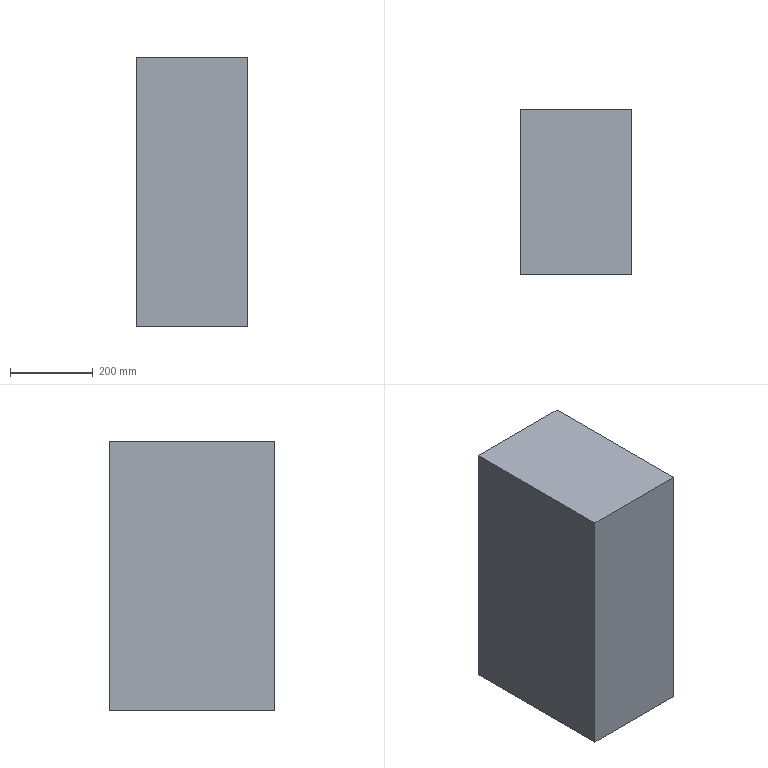Part | STEP file | kunzaxiang2 | 1 solid | 11 faces | box 270 x 400 x 650 mm | volume 28248000 mm3 | plane 11
STEP:
#1=CARTESIAN_POINT('',(0.,0.,0.));
#2=DIRECTION('',(0.,0.,1.));
#3=DIRECTION('',(1.,0.,0.));
#4=AXIS2_PLACEMENT_3D('',#1,#2,#3);
#5=CARTESIAN_POINT('',(135.,200.,325.));
#6=VERTEX_POINT('',#5);
#7=CARTESIAN_POINT('',(135.,200.,-325.));
#8=VERTEX_POINT('',#7);
#9=CARTESIAN_POINT('',(135.,200.,-325.));
#10=DIRECTION('',(0.,0.,-1.));
#11=VECTOR('',#10,1.);
#12=LINE('',#9,#11);
#13=CARTESIAN_POINT('',(0.,200.,0.));
#14=DIRECTION('',(0.,1.,0.));
#15=DIRECTION('',(0.,0.,1.));
#16=AXIS2_PLACEMENT_3D('',#13,#14,#15);
#17=PLANE('',#16);
#18=CARTESIAN_POINT('',(-325.,135.));
#19=DIRECTION('',(-1.,0.));
#20=VECTOR('',#19,1.);
#21=LINE('',#18,#20);
#22=(GEOMETRIC_REPRESENTATION_CONTEXT(2)PARAMETRIC_REPRESENTATION_CONTEXT()REPRESENTATION_CONTEXT('',''));
#23=DEFINITIONAL_REPRESENTATION('',(#21),#22);
#24=PCURVE('',#17,#23);
#25=CARTESIAN_POINT('',(135.,-200.,-325.));
#26=DIRECTION('',(1.,0.,0.));
#27=DIRECTION('',(0.,0.,-1.));
#28=AXIS2_PLACEMENT_3D('',#25,#26,#27);
#29=PLANE('',#28);
#30=CARTESIAN_POINT('',(0.,400.));
#31=DIRECTION('',(1.,0.));
#32=VECTOR('',#31,1.);
#33=LINE('',#30,#32);
#34=(GEOMETRIC_REPRESENTATION_CONTEXT(2)PARAMETRIC_REPRESENTATION_CONTEXT()REPRESENTATION_CONTEXT('',''));
#35=DEFINITIONAL_REPRESENTATION('',(#33),#34);
#36=PCURVE('',#29,#35);
#37=SURFACE_CURVE('',#12,(#24,#36),.PCURVE_S1.);
#38=EDGE_CURVE('',#6,#8,#37,.T.);
#39=ORIENTED_EDGE('',*,*,#38,.T.);
#40=CARTESIAN_POINT('',(-135.,200.,-325.));
#41=VERTEX_POINT('',#40);
#42=CARTESIAN_POINT('',(-135.,200.,-325.));
#43=DIRECTION('',(-1.,0.,0.));
#44=VECTOR('',#43,1.);
#45=LINE('',#42,#44);
#46=CARTESIAN_POINT('',(-325.,-135.));
#47=DIRECTION('',(0.,-1.));
#48=VECTOR('',#47,1.);
#49=LINE('',#46,#48);
#50=(GEOMETRIC_REPRESENTATION_CONTEXT(2)PARAMETRIC_REPRESENTATION_CONTEXT()REPRESENTATION_CONTEXT('',''));
#51=DEFINITIONAL_REPRESENTATION('',(#49),#50);
#52=PCURVE('',#17,#51);
#53=CARTESIAN_POINT('',(-135.,-200.,-325.));
#54=DIRECTION('',(0.,0.,-1.));
#55=DIRECTION('',(-1.,0.,0.));
#56=AXIS2_PLACEMENT_3D('',#53,#54,#55);
#57=PLANE('',#56);
#58=CARTESIAN_POINT('',(0.,400.));
#59=DIRECTION('',(1.,0.));
#60=VECTOR('',#59,1.);
#61=LINE('',#58,#60);
#62=(GEOMETRIC_REPRESENTATION_CONTEXT(2)PARAMETRIC_REPRESENTATION_CONTEXT()REPRESENTATION_CONTEXT('',''));
#63=DEFINITIONAL_REPRESENTATION('',(#61),#62);
#64=PCURVE('',#57,#63);
#65=SURFACE_CURVE('',#45,(#52,#64),.PCURVE_S1.);
#66=EDGE_CURVE('',#8,#41,#65,.T.);
#67=ORIENTED_EDGE('',*,*,#66,.T.);
#68=CARTESIAN_POINT('',(-135.,200.,325.));
#69=VERTEX_POINT('',#68);
#70=CARTESIAN_POINT('',(-135.,200.,-325.));
#71=DIRECTION('',(0.,0.,1.));
#72=VECTOR('',#71,1.);
#73=LINE('',#70,#72);
#74=CARTESIAN_POINT('',(-325.,-135.));
#75=DIRECTION('',(1.,0.));
#76=VECTOR('',#75,1.);
#77=LINE('',#74,#76);
#78=(GEOMETRIC_REPRESENTATION_CONTEXT(2)PARAMETRIC_REPRESENTATION_CONTEXT()REPRESENTATION_CONTEXT('',''));
#79=DEFINITIONAL_REPRESENTATION('',(#77),#78);
#80=PCURVE('',#17,#79);
#81=CARTESIAN_POINT('',(-135.,-200.,-325.));
#82=DIRECTION('',(-1.,0.,0.));
#83=DIRECTION('',(0.,0.,1.));
#84=AXIS2_PLACEMENT_3D('',#81,#82,#83);
#85=PLANE('',#84);
#86=CARTESIAN_POINT('',(0.,400.));
#87=DIRECTION('',(1.,0.));
#88=VECTOR('',#87,1.);
#89=LINE('',#86,#88);
#90=(GEOMETRIC_REPRESENTATION_CONTEXT(2)PARAMETRIC_REPRESENTATION_CONTEXT()REPRESENTATION_CONTEXT('',''));
#91=DEFINITIONAL_REPRESENTATION('',(#89),#90);
#92=PCURVE('',#85,#91);
#93=SURFACE_CURVE('',#73,(#80,#92),.PCURVE_S1.);
#94=EDGE_CURVE('',#41,#69,#93,.T.);
#95=ORIENTED_EDGE('',*,*,#94,.T.);
#96=CARTESIAN_POINT('',(-135.,200.,325.));
#97=DIRECTION('',(1.,0.,0.));
#98=VECTOR('',#97,1.);
#99=LINE('',#96,#98);
#100=CARTESIAN_POINT('',(325.,-135.));
#101=DIRECTION('',(0.,1.));
#102=VECTOR('',#101,1.);
#103=LINE('',#100,#102);
#104=(GEOMETRIC_REPRESENTATION_CONTEXT(2)PARAMETRIC_REPRESENTATION_CONTEXT()REPRESENTATION_CONTEXT('',''));
#105=DEFINITIONAL_REPRESENTATION('',(#103),#104);
#106=PCURVE('',#17,#105);
#107=CARTESIAN_POINT('',(-135.,-200.,325.));
#108=DIRECTION('',(0.,0.,1.));
#109=DIRECTION('',(1.,0.,0.));
#110=AXIS2_PLACEMENT_3D('',#107,#108,#109);
#111=PLANE('',#110);
#112=CARTESIAN_POINT('',(0.,400.));
#113=DIRECTION('',(1.,0.));
#114=VECTOR('',#113,1.);
#115=LINE('',#112,#114);
#116=(GEOMETRIC_REPRESENTATION_CONTEXT(2)PARAMETRIC_REPRESENTATION_CONTEXT()REPRESENTATION_CONTEXT('',''));
#117=DEFINITIONAL_REPRESENTATION('',(#115),#116);
#118=PCURVE('',#111,#117);
#119=SURFACE_CURVE('',#99,(#106,#118),.PCURVE_S1.);
#120=EDGE_CURVE('',#69,#6,#119,.T.);
#121=ORIENTED_EDGE('',*,*,#120,.T.);
#122=EDGE_LOOP('',(#39,#67,#95,#121));
#123=FACE_BOUND('',#122,.T.);
#124=CARTESIAN_POINT('',(120.,200.,-230.));
#125=VERTEX_POINT('',#124);
#126=CARTESIAN_POINT('',(-120.,200.,-230.));
#127=VERTEX_POINT('',#126);
#128=CARTESIAN_POINT('',(-120.,200.,-230.));
#129=DIRECTION('',(-1.,0.,0.));
#130=VECTOR('',#129,1.);
#131=LINE('',#128,#130);
#132=CARTESIAN_POINT('',(-230.,-120.));
#133=DIRECTION('',(0.,-1.));
#134=VECTOR('',#133,1.);
#135=LINE('',#132,#134);
#136=(GEOMETRIC_REPRESENTATION_CONTEXT(2)PARAMETRIC_REPRESENTATION_CONTEXT()REPRESENTATION_CONTEXT('',''));
#137=DEFINITIONAL_REPRESENTATION('',(#135),#136);
#138=PCURVE('',#17,#137);
#139=CARTESIAN_POINT('',(-120.,200.,-230.));
#140=DIRECTION('',(0.,0.,1.));
#141=DIRECTION('',(1.,0.,0.));
#142=AXIS2_PLACEMENT_3D('',#139,#140,#141);
#143=PLANE('',#142);
#144=CARTESIAN_POINT('',(0.,0.));
#145=DIRECTION('',(-1.,0.));
#146=VECTOR('',#145,1.);
#147=LINE('',#144,#146);
#148=(GEOMETRIC_REPRESENTATION_CONTEXT(2)PARAMETRIC_REPRESENTATION_CONTEXT()REPRESENTATION_CONTEXT('',''));
#149=DEFINITIONAL_REPRESENTATION('',(#147),#148);
#150=PCURVE('',#143,#149);
#151=SURFACE_CURVE('',#131,(#138,#150),.PCURVE_S1.);
#152=EDGE_CURVE('',#125,#127,#151,.T.);
#153=ORIENTED_EDGE('',*,*,#152,.F.);
#154=CARTESIAN_POINT('',(120.,200.,230.));
#155=VERTEX_POINT('',#154);
#156=CARTESIAN_POINT('',(120.,200.,-230.));
#157=DIRECTION('',(0.,0.,-1.));
#158=VECTOR('',#157,1.);
#159=LINE('',#156,#158);
#160=CARTESIAN_POINT('',(-230.,120.));
#161=DIRECTION('',(-1.,0.));
#162=VECTOR('',#161,1.);
#163=LINE('',#160,#162);
#164=(GEOMETRIC_REPRESENTATION_CONTEXT(2)PARAMETRIC_REPRESENTATION_CONTEXT()REPRESENTATION_CONTEXT('',''));
#165=DEFINITIONAL_REPRESENTATION('',(#163),#164);
#166=PCURVE('',#17,#165);
#167=CARTESIAN_POINT('',(120.,200.,-230.));
#168=DIRECTION('',(-1.,0.,0.));
#169=DIRECTION('',(0.,0.,1.));
#170=AXIS2_PLACEMENT_3D('',#167,#168,#169);
#171=PLANE('',#170);
#172=CARTESIAN_POINT('',(0.,0.));
#173=DIRECTION('',(-1.,0.));
#174=VECTOR('',#173,1.);
#175=LINE('',#172,#174);
#176=(GEOMETRIC_REPRESENTATION_CONTEXT(2)PARAMETRIC_REPRESENTATION_CONTEXT()REPRESENTATION_CONTEXT('',''));
#177=DEFINITIONAL_REPRESENTATION('',(#175),#176);
#178=PCURVE('',#171,#177);
#179=SURFACE_CURVE('',#159,(#166,#178),.PCURVE_S1.);
#180=EDGE_CURVE('',#155,#125,#179,.T.);
#181=ORIENTED_EDGE('',*,*,#180,.F.);
#182=CARTESIAN_POINT('',(-120.,200.,230.));
#183=VERTEX_POINT('',#182);
#184=CARTESIAN_POINT('',(-120.,200.,230.));
#185=DIRECTION('',(1.,0.,0.));
#186=VECTOR('',#185,1.);
#187=LINE('',#184,#186);
#188=CARTESIAN_POINT('',(230.,-120.));
#189=DIRECTION('',(0.,1.));
#190=VECTOR('',#189,1.);
#191=LINE('',#188,#190);
#192=(GEOMETRIC_REPRESENTATION_CONTEXT(2)PARAMETRIC_REPRESENTATION_CONTEXT()REPRESENTATION_CONTEXT('',''));
#193=DEFINITIONAL_REPRESENTATION('',(#191),#192);
#194=PCURVE('',#17,#193);
#195=CARTESIAN_POINT('',(-120.,200.,230.));
#196=DIRECTION('',(0.,0.,-1.));
#197=DIRECTION('',(-1.,0.,0.));
#198=AXIS2_PLACEMENT_3D('',#195,#196,#197);
#199=PLANE('',#198);
#200=CARTESIAN_POINT('',(0.,0.));
#201=DIRECTION('',(-1.,0.));
#202=VECTOR('',#201,1.);
#203=LINE('',#200,#202);
#204=(GEOMETRIC_REPRESENTATION_CONTEXT(2)PARAMETRIC_REPRESENTATION_CONTEXT()REPRESENTATION_CONTEXT('',''));
#205=DEFINITIONAL_REPRESENTATION('',(#203),#204);
#206=PCURVE('',#199,#205);
#207=SURFACE_CURVE('',#187,(#194,#206),.PCURVE_S1.);
#208=EDGE_CURVE('',#183,#155,#207,.T.);
#209=ORIENTED_EDGE('',*,*,#208,.F.);
#210=CARTESIAN_POINT('',(-120.,200.,-230.));
#211=DIRECTION('',(0.,0.,1.));
#212=VECTOR('',#211,1.);
#213=LINE('',#210,#212);
#214=CARTESIAN_POINT('',(-230.,-120.));
#215=DIRECTION('',(1.,0.));
#216=VECTOR('',#215,1.);
#217=LINE('',#214,#216);
#218=(GEOMETRIC_REPRESENTATION_CONTEXT(2)PARAMETRIC_REPRESENTATION_CONTEXT()REPRESENTATION_CONTEXT('',''));
#219=DEFINITIONAL_REPRESENTATION('',(#217),#218);
#220=PCURVE('',#17,#219);
#221=CARTESIAN_POINT('',(-120.,200.,-230.));
#222=DIRECTION('',(1.,0.,0.));
#223=DIRECTION('',(0.,0.,-1.));
#224=AXIS2_PLACEMENT_3D('',#221,#222,#223);
#225=PLANE('',#224);
#226=CARTESIAN_POINT('',(0.,0.));
#227=DIRECTION('',(-1.,0.));
#228=VECTOR('',#227,1.);
#229=LINE('',#226,#228);
#230=(GEOMETRIC_REPRESENTATION_CONTEXT(2)PARAMETRIC_REPRESENTATION_CONTEXT()REPRESENTATION_CONTEXT('',''));
#231=DEFINITIONAL_REPRESENTATION('',(#229),#230);
#232=PCURVE('',#225,#231);
#233=SURFACE_CURVE('',#213,(#220,#232),.PCURVE_S1.);
#234=EDGE_CURVE('',#127,#183,#233,.T.);
#235=ORIENTED_EDGE('',*,*,#234,.F.);
#236=EDGE_LOOP('',(#153,#181,#209,#235));
#237=FACE_BOUND('',#236,.T.);
#238=ADVANCED_FACE('',(#123,#237),#17,.T.);
#239=ORIENTED_EDGE('',*,*,#38,.F.);
#240=CARTESIAN_POINT('',(135.,-200.,325.));
#241=VERTEX_POINT('',#240);
#242=CARTESIAN_POINT('',(135.,-200.,325.));
#243=DIRECTION('',(0.,1.,0.));
#244=VECTOR('',#243,1.);
#245=LINE('',#242,#244);
#246=CARTESIAN_POINT('',(-650.,0.));
#247=DIRECTION('',(0.,1.));
#248=VECTOR('',#247,1.);
#249=LINE('',#246,#248);
#250=(GEOMETRIC_REPRESENTATION_CONTEXT(2)PARAMETRIC_REPRESENTATION_CONTEXT()REPRESENTATION_CONTEXT('',''));
#251=DEFINITIONAL_REPRESENTATION('',(#249),#250);
#252=PCURVE('',#29,#251);
#253=CARTESIAN_POINT('',(270.,0.));
#254=DIRECTION('',(0.,1.));
#255=VECTOR('',#254,1.);
#256=LINE('',#253,#255);
#257=(GEOMETRIC_REPRESENTATION_CONTEXT(2)PARAMETRIC_REPRESENTATION_CONTEXT()REPRESENTATION_CONTEXT('',''));
#258=DEFINITIONAL_REPRESENTATION('',(#256),#257);
#259=PCURVE('',#111,#258);
#260=SURFACE_CURVE('',#245,(#252,#259),.PCURVE_S1.);
#261=EDGE_CURVE('',#241,#6,#260,.T.);
#262=ORIENTED_EDGE('',*,*,#261,.F.);
#263=CARTESIAN_POINT('',(135.,-200.,-325.));
#264=VERTEX_POINT('',#263);
#265=CARTESIAN_POINT('',(135.,-200.,-325.));
#266=DIRECTION('',(0.,0.,-1.));
#267=VECTOR('',#266,1.);
#268=LINE('',#265,#267);
#269=CARTESIAN_POINT('',(0.,0.));
#270=DIRECTION('',(1.,0.));
#271=VECTOR('',#270,1.);
#272=LINE('',#269,#271);
#273=(GEOMETRIC_REPRESENTATION_CONTEXT(2)PARAMETRIC_REPRESENTATION_CONTEXT()REPRESENTATION_CONTEXT('',''));
#274=DEFINITIONAL_REPRESENTATION('',(#272),#273);
#275=PCURVE('',#29,#274);
#276=CARTESIAN_POINT('',(0.,-200.,0.));
#277=DIRECTION('',(0.,1.,0.));
#278=DIRECTION('',(0.,0.,1.));
#279=AXIS2_PLACEMENT_3D('',#276,#277,#278);
#280=PLANE('',#279);
#281=CARTESIAN_POINT('',(-325.,135.));
#282=DIRECTION('',(-1.,0.));
#283=VECTOR('',#282,1.);
#284=LINE('',#281,#283);
#285=(GEOMETRIC_REPRESENTATION_CONTEXT(2)PARAMETRIC_REPRESENTATION_CONTEXT()REPRESENTATION_CONTEXT('',''));
#286=DEFINITIONAL_REPRESENTATION('',(#284),#285);
#287=PCURVE('',#280,#286);
#288=SURFACE_CURVE('',#268,(#275,#287),.PCURVE_S1.);
#289=EDGE_CURVE('',#241,#264,#288,.T.);
#290=ORIENTED_EDGE('',*,*,#289,.T.);
#291=CARTESIAN_POINT('',(135.,-200.,-325.));
#292=DIRECTION('',(0.,1.,0.));
#293=VECTOR('',#292,1.);
#294=LINE('',#291,#293);
#295=CARTESIAN_POINT('',(0.,0.));
#296=DIRECTION('',(0.,1.));
#297=VECTOR('',#296,1.);
#298=LINE('',#295,#297);
#299=(GEOMETRIC_REPRESENTATION_CONTEXT(2)PARAMETRIC_REPRESENTATION_CONTEXT()REPRESENTATION_CONTEXT('',''));
#300=DEFINITIONAL_REPRESENTATION('',(#298),#299);
#301=PCURVE('',#29,#300);
#302=CARTESIAN_POINT('',(-270.,0.));
#303=DIRECTION('',(0.,1.));
#304=VECTOR('',#303,1.);
#305=LINE('',#302,#304);
#306=(GEOMETRIC_REPRESENTATION_CONTEXT(2)PARAMETRIC_REPRESENTATION_CONTEXT()REPRESENTATION_CONTEXT('',''));
#307=DEFINITIONAL_REPRESENTATION('',(#305),#306);
#308=PCURVE('',#57,#307);
#309=SURFACE_CURVE('',#294,(#301,#308),.PCURVE_S1.);
#310=EDGE_CURVE('',#264,#8,#309,.T.);
#311=ORIENTED_EDGE('',*,*,#310,.T.);
#312=EDGE_LOOP('',(#239,#262,#290,#311));
#313=FACE_BOUND('',#312,.T.);
#314=ADVANCED_FACE('',(#313),#29,.T.);
#315=ORIENTED_EDGE('',*,*,#120,.F.);
#316=CARTESIAN_POINT('',(-135.,-200.,325.));
#317=VERTEX_POINT('',#316);
#318=CARTESIAN_POINT('',(-135.,-200.,325.));
#319=DIRECTION('',(0.,1.,0.));
#320=VECTOR('',#319,1.);
#321=LINE('',#318,#320);
#322=CARTESIAN_POINT('',(0.,0.));
#323=DIRECTION('',(0.,1.));
#324=VECTOR('',#323,1.);
#325=LINE('',#322,#324);
#326=(GEOMETRIC_REPRESENTATION_CONTEXT(2)PARAMETRIC_REPRESENTATION_CONTEXT()REPRESENTATION_CONTEXT('',''));
#327=DEFINITIONAL_REPRESENTATION('',(#325),#326);
#328=PCURVE('',#111,#327);
#329=CARTESIAN_POINT('',(650.,0.));
#330=DIRECTION('',(0.,1.));
#331=VECTOR('',#330,1.);
#332=LINE('',#329,#331);
#333=(GEOMETRIC_REPRESENTATION_CONTEXT(2)PARAMETRIC_REPRESENTATION_CONTEXT()REPRESENTATION_CONTEXT('',''));
#334=DEFINITIONAL_REPRESENTATION('',(#332),#333);
#335=PCURVE('',#85,#334);
#336=SURFACE_CURVE('',#321,(#328,#335),.PCURVE_S1.);
#337=EDGE_CURVE('',#317,#69,#336,.T.);
#338=ORIENTED_EDGE('',*,*,#337,.F.);
#339=CARTESIAN_POINT('',(-135.,-200.,325.));
#340=DIRECTION('',(1.,0.,0.));
#341=VECTOR('',#340,1.);
#342=LINE('',#339,#341);
#343=CARTESIAN_POINT('',(0.,0.));
#344=DIRECTION('',(1.,0.));
#345=VECTOR('',#344,1.);
#346=LINE('',#343,#345);
#347=(GEOMETRIC_REPRESENTATION_CONTEXT(2)PARAMETRIC_REPRESENTATION_CONTEXT()REPRESENTATION_CONTEXT('',''));
#348=DEFINITIONAL_REPRESENTATION('',(#346),#347);
#349=PCURVE('',#111,#348);
#350=CARTESIAN_POINT('',(325.,-135.));
#351=DIRECTION('',(0.,1.));
#352=VECTOR('',#351,1.);
#353=LINE('',#350,#352);
#354=(GEOMETRIC_REPRESENTATION_CONTEXT(2)PARAMETRIC_REPRESENTATION_CONTEXT()REPRESENTATION_CONTEXT('',''));
#355=DEFINITIONAL_REPRESENTATION('',(#353),#354);
#356=PCURVE('',#280,#355);
#357=SURFACE_CURVE('',#342,(#349,#356),.PCURVE_S1.);
#358=EDGE_CURVE('',#317,#241,#357,.T.);
#359=ORIENTED_EDGE('',*,*,#358,.T.);
#360=ORIENTED_EDGE('',*,*,#261,.T.);
#361=EDGE_LOOP('',(#315,#338,#359,#360));
#362=FACE_BOUND('',#361,.T.);
#363=ADVANCED_FACE('',(#362),#111,.T.);
#364=ORIENTED_EDGE('',*,*,#94,.F.);
#365=CARTESIAN_POINT('',(-135.,-200.,-325.));
#366=VERTEX_POINT('',#365);
#367=CARTESIAN_POINT('',(-135.,-200.,-325.));
#368=DIRECTION('',(0.,1.,0.));
#369=VECTOR('',#368,1.);
#370=LINE('',#367,#369);
#371=CARTESIAN_POINT('',(0.,0.));
#372=DIRECTION('',(0.,1.));
#373=VECTOR('',#372,1.);
#374=LINE('',#371,#373);
#375=(GEOMETRIC_REPRESENTATION_CONTEXT(2)PARAMETRIC_REPRESENTATION_CONTEXT()REPRESENTATION_CONTEXT('',''));
#376=DEFINITIONAL_REPRESENTATION('',(#374),#375);
#377=PCURVE('',#85,#376);
#378=CARTESIAN_POINT('',(0.,0.));
#379=DIRECTION('',(0.,1.));
#380=VECTOR('',#379,1.);
#381=LINE('',#378,#380);
#382=(GEOMETRIC_REPRESENTATION_CONTEXT(2)PARAMETRIC_REPRESENTATION_CONTEXT()REPRESENTATION_CONTEXT('',''));
#383=DEFINITIONAL_REPRESENTATION('',(#381),#382);
#384=PCURVE('',#57,#383);
#385=SURFACE_CURVE('',#370,(#377,#384),.PCURVE_S1.);
#386=EDGE_CURVE('',#366,#41,#385,.T.);
#387=ORIENTED_EDGE('',*,*,#386,.F.);
#388=CARTESIAN_POINT('',(-135.,-200.,-325.));
#389=DIRECTION('',(0.,0.,1.));
#390=VECTOR('',#389,1.);
#391=LINE('',#388,#390);
#392=CARTESIAN_POINT('',(0.,0.));
#393=DIRECTION('',(1.,0.));
#394=VECTOR('',#393,1.);
#395=LINE('',#392,#394);
#396=(GEOMETRIC_REPRESENTATION_CONTEXT(2)PARAMETRIC_REPRESENTATION_CONTEXT()REPRESENTATION_CONTEXT('',''));
#397=DEFINITIONAL_REPRESENTATION('',(#395),#396);
#398=PCURVE('',#85,#397);
#399=CARTESIAN_POINT('',(-325.,-135.));
#400=DIRECTION('',(1.,0.));
#401=VECTOR('',#400,1.);
#402=LINE('',#399,#401);
#403=(GEOMETRIC_REPRESENTATION_CONTEXT(2)PARAMETRIC_REPRESENTATION_CONTEXT()REPRESENTATION_CONTEXT('',''));
#404=DEFINITIONAL_REPRESENTATION('',(#402),#403);
#405=PCURVE('',#280,#404);
#406=SURFACE_CURVE('',#391,(#398,#405),.PCURVE_S1.);
#407=EDGE_CURVE('',#366,#317,#406,.T.);
#408=ORIENTED_EDGE('',*,*,#407,.T.);
#409=ORIENTED_EDGE('',*,*,#337,.T.);
#410=EDGE_LOOP('',(#364,#387,#408,#409));
#411=FACE_BOUND('',#410,.T.);
#412=ADVANCED_FACE('',(#411),#85,.T.);
#413=ORIENTED_EDGE('',*,*,#66,.F.);
#414=ORIENTED_EDGE('',*,*,#310,.F.);
#415=CARTESIAN_POINT('',(-135.,-200.,-325.));
#416=DIRECTION('',(-1.,0.,0.));
#417=VECTOR('',#416,1.);
#418=LINE('',#415,#417);
#419=CARTESIAN_POINT('',(0.,0.));
#420=DIRECTION('',(1.,0.));
#421=VECTOR('',#420,1.);
#422=LINE('',#419,#421);
#423=(GEOMETRIC_REPRESENTATION_CONTEXT(2)PARAMETRIC_REPRESENTATION_CONTEXT()REPRESENTATION_CONTEXT('',''));
#424=DEFINITIONAL_REPRESENTATION('',(#422),#423);
#425=PCURVE('',#57,#424);
#426=CARTESIAN_POINT('',(-325.,-135.));
#427=DIRECTION('',(0.,-1.));
#428=VECTOR('',#427,1.);
#429=LINE('',#426,#428);
#430=(GEOMETRIC_REPRESENTATION_CONTEXT(2)PARAMETRIC_REPRESENTATION_CONTEXT()REPRESENTATION_CONTEXT('',''));
#431=DEFINITIONAL_REPRESENTATION('',(#429),#430);
#432=PCURVE('',#280,#431);
#433=SURFACE_CURVE('',#418,(#425,#432),.PCURVE_S1.);
#434=EDGE_CURVE('',#264,#366,#433,.T.);
#435=ORIENTED_EDGE('',*,*,#434,.T.);
#436=ORIENTED_EDGE('',*,*,#386,.T.);
#437=EDGE_LOOP('',(#413,#414,#435,#436));
#438=FACE_BOUND('',#437,.T.);
#439=ADVANCED_FACE('',(#438),#57,.T.);
#440=ORIENTED_EDGE('',*,*,#289,.F.);
#441=ORIENTED_EDGE('',*,*,#358,.F.);
#442=ORIENTED_EDGE('',*,*,#407,.F.);
#443=ORIENTED_EDGE('',*,*,#434,.F.);
#444=EDGE_LOOP('',(#440,#441,#442,#443));
#445=FACE_BOUND('',#444,.T.);
#446=ADVANCED_FACE('',(#445),#280,.F.);
#447=CARTESIAN_POINT('',(120.,-180.,230.));
#448=VERTEX_POINT('',#447);
#449=CARTESIAN_POINT('',(120.,200.,230.));
#450=DIRECTION('',(0.,-1.,0.));
#451=VECTOR('',#450,1.);
#452=LINE('',#449,#451);
#453=CARTESIAN_POINT('',(460.,0.));
#454=DIRECTION('',(0.,-1.));
#455=VECTOR('',#454,1.);
#456=LINE('',#453,#455);
#457=(GEOMETRIC_REPRESENTATION_CONTEXT(2)PARAMETRIC_REPRESENTATION_CONTEXT()REPRESENTATION_CONTEXT('',''));
#458=DEFINITIONAL_REPRESENTATION('',(#456),#457);
#459=PCURVE('',#171,#458);
#460=CARTESIAN_POINT('',(-240.,0.));
#461=DIRECTION('',(0.,-1.));
#462=VECTOR('',#461,1.);
#463=LINE('',#460,#462);
#464=(GEOMETRIC_REPRESENTATION_CONTEXT(2)PARAMETRIC_REPRESENTATION_CONTEXT()REPRESENTATION_CONTEXT('',''));
#465=DEFINITIONAL_REPRESENTATION('',(#463),#464);
#466=PCURVE('',#199,#465);
#467=SURFACE_CURVE('',#452,(#459,#466),.PCURVE_S1.);
#468=EDGE_CURVE('',#155,#448,#467,.T.);
#469=ORIENTED_EDGE('',*,*,#468,.F.);
#470=ORIENTED_EDGE('',*,*,#180,.T.);
#471=CARTESIAN_POINT('',(120.,-180.,-230.));
#472=VERTEX_POINT('',#471);
#473=CARTESIAN_POINT('',(120.,200.,-230.));
#474=DIRECTION('',(0.,-1.,0.));
#475=VECTOR('',#474,1.);
#476=LINE('',#473,#475);
#477=CARTESIAN_POINT('',(0.,0.));
#478=DIRECTION('',(0.,-1.));
#479=VECTOR('',#478,1.);
#480=LINE('',#477,#479);
#481=(GEOMETRIC_REPRESENTATION_CONTEXT(2)PARAMETRIC_REPRESENTATION_CONTEXT()REPRESENTATION_CONTEXT('',''));
#482=DEFINITIONAL_REPRESENTATION('',(#480),#481);
#483=PCURVE('',#171,#482);
#484=CARTESIAN_POINT('',(240.,0.));
#485=DIRECTION('',(0.,-1.));
#486=VECTOR('',#485,1.);
#487=LINE('',#484,#486);
#488=(GEOMETRIC_REPRESENTATION_CONTEXT(2)PARAMETRIC_REPRESENTATION_CONTEXT()REPRESENTATION_CONTEXT('',''));
#489=DEFINITIONAL_REPRESENTATION('',(#487),#488);
#490=PCURVE('',#143,#489);
#491=SURFACE_CURVE('',#476,(#483,#490),.PCURVE_S1.);
#492=EDGE_CURVE('',#125,#472,#491,.T.);
#493=ORIENTED_EDGE('',*,*,#492,.T.);
#494=CARTESIAN_POINT('',(120.,-180.,-230.));
#495=DIRECTION('',(0.,0.,-1.));
#496=VECTOR('',#495,1.);
#497=LINE('',#494,#496);
#498=CARTESIAN_POINT('',(0.,-380.));
#499=DIRECTION('',(-1.,0.));
#500=VECTOR('',#499,1.);
#501=LINE('',#498,#500);
#502=(GEOMETRIC_REPRESENTATION_CONTEXT(2)PARAMETRIC_REPRESENTATION_CONTEXT()REPRESENTATION_CONTEXT('',''));
#503=DEFINITIONAL_REPRESENTATION('',(#501),#502);
#504=PCURVE('',#171,#503);
#505=CARTESIAN_POINT('',(0.,-180.,0.));
#506=DIRECTION('',(0.,1.,0.));
#507=DIRECTION('',(0.,0.,1.));
#508=AXIS2_PLACEMENT_3D('',#505,#506,#507);
#509=PLANE('',#508);
#510=CARTESIAN_POINT('',(-230.,120.));
#511=DIRECTION('',(-1.,0.));
#512=VECTOR('',#511,1.);
#513=LINE('',#510,#512);
#514=(GEOMETRIC_REPRESENTATION_CONTEXT(2)PARAMETRIC_REPRESENTATION_CONTEXT()REPRESENTATION_CONTEXT('',''));
#515=DEFINITIONAL_REPRESENTATION('',(#513),#514);
#516=PCURVE('',#509,#515);
#517=SURFACE_CURVE('',#497,(#504,#516),.PCURVE_S1.);
#518=EDGE_CURVE('',#448,#472,#517,.T.);
#519=ORIENTED_EDGE('',*,*,#518,.F.);
#520=EDGE_LOOP('',(#469,#470,#493,#519));
#521=FACE_BOUND('',#520,.T.);
#522=ADVANCED_FACE('',(#521),#171,.T.);
#523=ORIENTED_EDGE('',*,*,#492,.F.);
#524=ORIENTED_EDGE('',*,*,#152,.T.);
#525=CARTESIAN_POINT('',(-120.,-180.,-230.));
#526=VERTEX_POINT('',#525);
#527=CARTESIAN_POINT('',(-120.,200.,-230.));
#528=DIRECTION('',(0.,-1.,0.));
#529=VECTOR('',#528,1.);
#530=LINE('',#527,#529);
#531=CARTESIAN_POINT('',(0.,0.));
#532=DIRECTION('',(0.,-1.));
#533=VECTOR('',#532,1.);
#534=LINE('',#531,#533);
#535=(GEOMETRIC_REPRESENTATION_CONTEXT(2)PARAMETRIC_REPRESENTATION_CONTEXT()REPRESENTATION_CONTEXT('',''));
#536=DEFINITIONAL_REPRESENTATION('',(#534),#535);
#537=PCURVE('',#143,#536);
#538=CARTESIAN_POINT('',(0.,0.));
#539=DIRECTION('',(0.,-1.));
#540=VECTOR('',#539,1.);
#541=LINE('',#538,#540);
#542=(GEOMETRIC_REPRESENTATION_CONTEXT(2)PARAMETRIC_REPRESENTATION_CONTEXT()REPRESENTATION_CONTEXT('',''));
#543=DEFINITIONAL_REPRESENTATION('',(#541),#542);
#544=PCURVE('',#225,#543);
#545=SURFACE_CURVE('',#530,(#537,#544),.PCURVE_S1.);
#546=EDGE_CURVE('',#127,#526,#545,.T.);
#547=ORIENTED_EDGE('',*,*,#546,.T.);
#548=CARTESIAN_POINT('',(-120.,-180.,-230.));
#549=DIRECTION('',(-1.,0.,0.));
#550=VECTOR('',#549,1.);
#551=LINE('',#548,#550);
#552=CARTESIAN_POINT('',(0.,-380.));
#553=DIRECTION('',(-1.,0.));
#554=VECTOR('',#553,1.);
#555=LINE('',#552,#554);
#556=(GEOMETRIC_REPRESENTATION_CONTEXT(2)PARAMETRIC_REPRESENTATION_CONTEXT()REPRESENTATION_CONTEXT('',''));
#557=DEFINITIONAL_REPRESENTATION('',(#555),#556);
#558=PCURVE('',#143,#557);
#559=CARTESIAN_POINT('',(-230.,-120.));
#560=DIRECTION('',(0.,-1.));
#561=VECTOR('',#560,1.);
#562=LINE('',#559,#561);
#563=(GEOMETRIC_REPRESENTATION_CONTEXT(2)PARAMETRIC_REPRESENTATION_CONTEXT()REPRESENTATION_CONTEXT('',''));
#564=DEFINITIONAL_REPRESENTATION('',(#562),#563);
#565=PCURVE('',#509,#564);
#566=SURFACE_CURVE('',#551,(#558,#565),.PCURVE_S1.);
#567=EDGE_CURVE('',#472,#526,#566,.T.);
#568=ORIENTED_EDGE('',*,*,#567,.F.);
#569=EDGE_LOOP('',(#523,#524,#547,#568));
#570=FACE_BOUND('',#569,.T.);
#571=ADVANCED_FACE('',(#570),#143,.T.);
#572=ORIENTED_EDGE('',*,*,#546,.F.);
#573=ORIENTED_EDGE('',*,*,#234,.T.);
#574=CARTESIAN_POINT('',(-120.,-180.,230.));
#575=VERTEX_POINT('',#574);
#576=CARTESIAN_POINT('',(-120.,200.,230.));
#577=DIRECTION('',(0.,-1.,0.));
#578=VECTOR('',#577,1.);
#579=LINE('',#576,#578);
#580=CARTESIAN_POINT('',(-460.,0.));
#581=DIRECTION('',(0.,-1.));
#582=VECTOR('',#581,1.);
#583=LINE('',#580,#582);
#584=(GEOMETRIC_REPRESENTATION_CONTEXT(2)PARAMETRIC_REPRESENTATION_CONTEXT()REPRESENTATION_CONTEXT('',''));
#585=DEFINITIONAL_REPRESENTATION('',(#583),#584);
#586=PCURVE('',#225,#585);
#587=CARTESIAN_POINT('',(0.,0.));
#588=DIRECTION('',(0.,-1.));
#589=VECTOR('',#588,1.);
#590=LINE('',#587,#589);
#591=(GEOMETRIC_REPRESENTATION_CONTEXT(2)PARAMETRIC_REPRESENTATION_CONTEXT()REPRESENTATION_CONTEXT('',''));
#592=DEFINITIONAL_REPRESENTATION('',(#590),#591);
#593=PCURVE('',#199,#592);
#594=SURFACE_CURVE('',#579,(#586,#593),.PCURVE_S1.);
#595=EDGE_CURVE('',#183,#575,#594,.T.);
#596=ORIENTED_EDGE('',*,*,#595,.T.);
#597=CARTESIAN_POINT('',(-120.,-180.,-230.));
#598=DIRECTION('',(0.,0.,1.));
#599=VECTOR('',#598,1.);
#600=LINE('',#597,#599);
#601=CARTESIAN_POINT('',(0.,-380.));
#602=DIRECTION('',(-1.,0.));
#603=VECTOR('',#602,1.);
#604=LINE('',#601,#603);
#605=(GEOMETRIC_REPRESENTATION_CONTEXT(2)PARAMETRIC_REPRESENTATION_CONTEXT()REPRESENTATION_CONTEXT('',''));
#606=DEFINITIONAL_REPRESENTATION('',(#604),#605);
#607=PCURVE('',#225,#606);
#608=CARTESIAN_POINT('',(-230.,-120.));
#609=DIRECTION('',(1.,0.));
#610=VECTOR('',#609,1.);
#611=LINE('',#608,#610);
#612=(GEOMETRIC_REPRESENTATION_CONTEXT(2)PARAMETRIC_REPRESENTATION_CONTEXT()REPRESENTATION_CONTEXT('',''));
#613=DEFINITIONAL_REPRESENTATION('',(#611),#612);
#614=PCURVE('',#509,#613);
#615=SURFACE_CURVE('',#600,(#607,#614),.PCURVE_S1.);
#616=EDGE_CURVE('',#526,#575,#615,.T.);
#617=ORIENTED_EDGE('',*,*,#616,.F.);
#618=EDGE_LOOP('',(#572,#573,#596,#617));
#619=FACE_BOUND('',#618,.T.);
#620=ADVANCED_FACE('',(#619),#225,.T.);
#621=ORIENTED_EDGE('',*,*,#595,.F.);
#622=ORIENTED_EDGE('',*,*,#208,.T.);
#623=ORIENTED_EDGE('',*,*,#468,.T.);
#624=CARTESIAN_POINT('',(-120.,-180.,230.));
#625=DIRECTION('',(1.,0.,0.));
#626=VECTOR('',#625,1.);
#627=LINE('',#624,#626);
#628=CARTESIAN_POINT('',(0.,-380.));
#629=DIRECTION('',(-1.,0.));
#630=VECTOR('',#629,1.);
#631=LINE('',#628,#630);
#632=(GEOMETRIC_REPRESENTATION_CONTEXT(2)PARAMETRIC_REPRESENTATION_CONTEXT()REPRESENTATION_CONTEXT('',''));
#633=DEFINITIONAL_REPRESENTATION('',(#631),#632);
#634=PCURVE('',#199,#633);
#635=CARTESIAN_POINT('',(230.,-120.));
#636=DIRECTION('',(0.,1.));
#637=VECTOR('',#636,1.);
#638=LINE('',#635,#637);
#639=(GEOMETRIC_REPRESENTATION_CONTEXT(2)PARAMETRIC_REPRESENTATION_CONTEXT()REPRESENTATION_CONTEXT('',''));
#640=DEFINITIONAL_REPRESENTATION('',(#638),#639);
#641=PCURVE('',#509,#640);
#642=SURFACE_CURVE('',#627,(#634,#641),.PCURVE_S1.);
#643=EDGE_CURVE('',#575,#448,#642,.T.);
#644=ORIENTED_EDGE('',*,*,#643,.F.);
#645=EDGE_LOOP('',(#621,#622,#623,#644));
#646=FACE_BOUND('',#645,.T.);
#647=ADVANCED_FACE('',(#646),#199,.T.);
#648=ORIENTED_EDGE('',*,*,#518,.T.);
#649=ORIENTED_EDGE('',*,*,#567,.T.);
#650=ORIENTED_EDGE('',*,*,#616,.T.);
#651=ORIENTED_EDGE('',*,*,#643,.T.);
#652=EDGE_LOOP('',(#648,#649,#650,#651));
#653=FACE_BOUND('',#652,.T.);
#654=ADVANCED_FACE('',(#653),#509,.T.);
#655=CLOSED_SHELL('',(#238,#314,#363,#412,#439,#446,#522,#571,#620,#647,#654));
#656=MANIFOLD_SOLID_BREP('',#655);
#657=(LENGTH_UNIT()NAMED_UNIT(*)SI_UNIT(.MILLI.,.METRE.));
#658=UNCERTAINTY_MEASURE_WITH_UNIT(LENGTH_MEASURE(0.0000001),#657,'','');
#659=(NAMED_UNIT(*)PLANE_ANGLE_UNIT()SI_UNIT($,.RADIAN.));
#660=(NAMED_UNIT(*)SI_UNIT($,.STERADIAN.)SOLID_ANGLE_UNIT());
#661=(GEOMETRIC_REPRESENTATION_CONTEXT(3)GLOBAL_UNCERTAINTY_ASSIGNED_CONTEXT((#658))GLOBAL_UNIT_ASSIGNED_CONTEXT((#657,#659,#660))REPRESENTATION_CONTEXT('',''));
#662=ADVANCED_BREP_SHAPE_REPRESENTATION('',(#4,#656),#661);